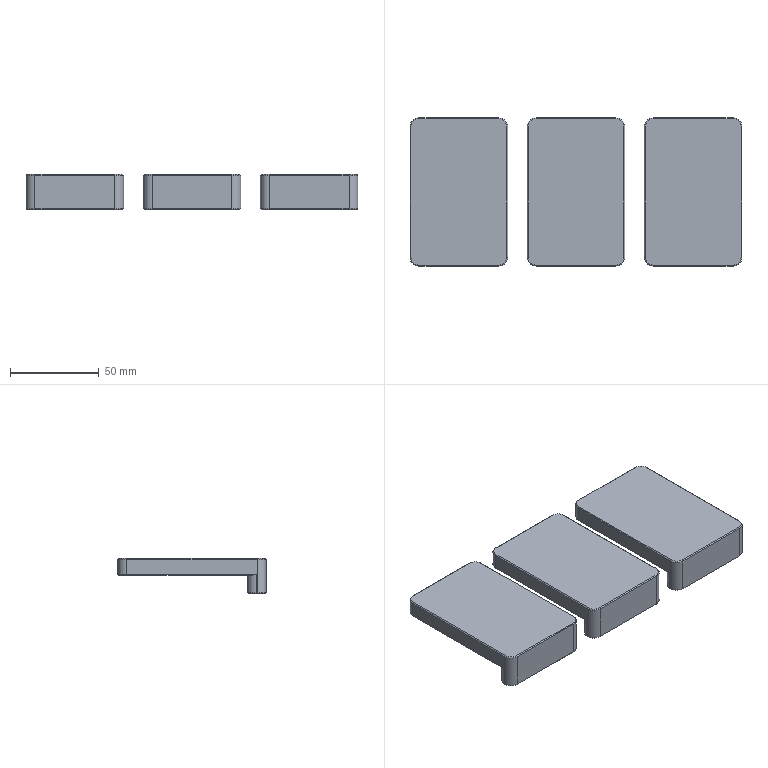NC program | NX | posted with a generic post | part box 187 x 83.5 x 20 mm
Lines 5413 to 5666 of 5666:
(ZLEVEL_PROFILE_COPY_1_COPY , TOOL : D10JING)
N10818 T14 M6
N10820 G54
N10822 G17 G0 G90 X33.89 Y39.594 S9500 M3
N10824 G43 Z30. H14
N10826 Z1.5
N10828 G94 G1 X34.613 Y41.399 Z1.398 F1000.
N10830 X35.728 Y43.09 Z1.292
N10832 X37.16 Y44.522 Z1.186
N10834 X38.851 Y45.637 Z1.08
N10836 X40.731 Y46.39 Z0.973
N10838 X42.725 Y46.75 Z0.867
N10840 X89.275 Z-1.572
N10842 X91.269 Y46.39 Z-1.678
N10844 X93.149 Y45.637 Z-1.785
N10846 X94.84 Y44.522 Z-1.891
N10848 X96.272 Y43.09 Z-1.997
N10850 X97.387 Y41.399 Z-2.103
N10852 X98.14 Y39.519 Z-2.209
N10854 X98.5 Y37.525 Z-2.315
N10856 Y-37.525 Z-6.249
N10858 X98.14 Y-39.519 Z-6.355
N10860 X97.387 Y-41.399 Z-6.461
N10862 X96.272 Y-43.09 Z-6.567
N10864 X94.84 Y-44.522 Z-6.673
N10866 X93.149 Y-45.637 Z-6.779
N10868 X91.269 Y-46.39 Z-6.886
N10870 X89.275 Y-46.75 Z-6.992
N10872 X42.725 Z-9.431
N10874 X40.731 Y-46.39 Z-9.537
N10876 X38.851 Y-45.637 Z-9.644
N10878 X37.16 Y-44.522 Z-9.75
N10880 X35.728 Y-43.09 Z-9.856
N10882 X34.613 Y-41.399 Z-9.962
N10884 X33.86 Y-39.519 Z-10.068
N10886 X33.5 Y-37.525 Z-10.174
N10888 Y37.525 Z-14.108
N10890 X33.86 Y39.519 Z-14.214
N10892 X34.613 Y41.399 Z-14.32
N10894 X35.728 Y43.09 Z-14.426
N10896 X37.16 Y44.522 Z-14.532
N10898 X38.851 Y45.637 Z-14.638
N10900 X40.731 Y46.39 Z-14.745
N10902 X42.725 Y46.75 Z-14.851
N10904 X89.275 Z-17.29
N10906 X91.269 Y46.39 Z-17.396
N10908 X93.149 Y45.637 Z-17.503
N10910 X94.84 Y44.522 Z-17.609
N10912 X96.272 Y43.09 Z-17.715
N10914 X97.387 Y41.399 Z-17.821
N10916 X98.14 Y39.519 Z-17.927
N10918 X98.5 Y37.525 Z-18.033
N10920 Y0. Z-20.
N10922 Y-36.75 F1200.
N10924 G2 X88.5 Y-46.75 R10.
N10926 G1 X43.5
N10928 G2 X33.5 Y-36.75 R10.
N10930 G1 Y36.75
N10932 G2 X43.5 Y46.75 R10.
N10934 G1 X88.5
N10936 G2 X98.5 Y36.75 R10.
N10938 G1 Y0.
N10940 G3 X99. Y-0.866 R1.
N10942 G1 X99.5 Y-1.155
N10944 Z-19.
N10946 G0 Z53.
N10948 X-33.89 Y-39.594
N10950 Z1.5
N10952 G1 X-34.613 Y-41.399 Z1.398 F1000.
N10954 X-35.728 Y-43.09 Z1.292
N10956 X-37.16 Y-44.522 Z1.186
N10958 X-38.851 Y-45.637 Z1.08
N10960 X-40.731 Y-46.39 Z0.973
N10962 X-42.725 Y-46.75 Z0.867
N10964 X-89.275 Z-1.572
N10966 X-91.269 Y-46.39 Z-1.678
N10968 X-93.149 Y-45.637 Z-1.785
N10970 X-94.84 Y-44.522 Z-1.891
N10972 X-96.272 Y-43.09 Z-1.997
N10974 X-97.387 Y-41.399 Z-2.103
N10976 X-98.14 Y-39.519 Z-2.209
N10978 X-98.5 Y-37.525 Z-2.315
N10980 Y37.525 Z-6.249
N10982 X-98.14 Y39.519 Z-6.355
N10984 X-97.387 Y41.399 Z-6.461
N10986 X-96.272 Y43.09 Z-6.567
N10988 X-94.84 Y44.522 Z-6.673
N10990 X-93.149 Y45.637 Z-6.779
N10992 X-91.269 Y46.39 Z-6.886
N10994 X-89.275 Y46.75 Z-6.992
N10996 X-42.725 Z-9.431
N10998 X-40.731 Y46.39 Z-9.537
N11000 X-38.851 Y45.637 Z-9.644
N11002 X-37.16 Y44.522 Z-9.75
N11004 X-35.728 Y43.09 Z-9.856
N11006 X-34.613 Y41.399 Z-9.962
N11008 X-33.86 Y39.519 Z-10.068
N11010 X-33.5 Y37.525 Z-10.174
N11012 Y-37.525 Z-14.108
N11014 X-33.86 Y-39.519 Z-14.214
N11016 X-34.613 Y-41.399 Z-14.32
N11018 X-35.728 Y-43.09 Z-14.426
N11020 X-37.16 Y-44.522 Z-14.532
N11022 X-38.851 Y-45.637 Z-14.638
N11024 X-40.731 Y-46.39 Z-14.745
N11026 X-42.725 Y-46.75 Z-14.851
N11028 X-89.275 Z-17.29
N11030 X-91.269 Y-46.39 Z-17.396
N11032 X-93.149 Y-45.637 Z-17.503
N11034 X-94.84 Y-44.522 Z-17.609
N11036 X-96.272 Y-43.09 Z-17.715
N11038 X-97.387 Y-41.399 Z-17.821
N11040 X-98.14 Y-39.519 Z-17.927
N11042 X-98.5 Y-37.525 Z-18.033
N11044 Y0. Z-20.
N11046 Y36.75 F1200.
N11048 G2 X-88.5 Y46.75 R10.
N11050 G1 X-43.5
N11052 G2 X-33.5 Y36.75 R10.
N11054 G1 Y-36.75
N11056 G2 X-43.5 Y-46.75 R10.
N11058 G1 X-88.5
N11060 G2 X-98.5 Y-36.75 R10.
N11062 G1 Y0.
N11064 G3 X-99. Y0.866 R1.
N11066 G1 X-99.5 Y1.155
N11068 Z-19.
N11070 G0 Z53.
N11072 X32.11 Y-39.594
N11074 Z1.5
N11076 G1 X31.387 Y-41.399 Z1.398 F1000.
N11078 X30.272 Y-43.09 Z1.292
N11080 X28.84 Y-44.522 Z1.186
N11082 X27.149 Y-45.637 Z1.08
N11084 X25.269 Y-46.39 Z0.973
N11086 X23.275 Y-46.75 Z0.867
N11088 X-23.275 Z-1.572
N11090 X-25.269 Y-46.39 Z-1.678
N11092 X-27.149 Y-45.637 Z-1.785
N11094 X-28.84 Y-44.522 Z-1.891
N11096 X-30.272 Y-43.09 Z-1.997
N11098 X-31.387 Y-41.399 Z-2.103
N11100 X-32.14 Y-39.519 Z-2.209
N11102 X-32.5 Y-37.525 Z-2.315
N11104 Y37.525 Z-6.249
N11106 X-32.14 Y39.519 Z-6.355
N11108 X-31.387 Y41.399 Z-6.461
N11110 X-30.272 Y43.09 Z-6.567
N11112 X-28.84 Y44.522 Z-6.673
N11114 X-27.149 Y45.637 Z-6.779
N11116 X-25.269 Y46.39 Z-6.886
N11118 X-23.275 Y46.75 Z-6.992
N11120 X23.275 Z-9.431
N11122 X25.269 Y46.39 Z-9.537
N11124 X27.149 Y45.637 Z-9.644
N11126 X28.84 Y44.522 Z-9.75
N11128 X30.272 Y43.09 Z-9.856
N11130 X31.387 Y41.399 Z-9.962
N11132 X32.14 Y39.519 Z-10.068
N11134 X32.5 Y37.525 Z-10.174
N11136 Y-37.525 Z-14.108
N11138 X32.14 Y-39.519 Z-14.214
N11140 X31.387 Y-41.399 Z-14.32
N11142 X30.272 Y-43.09 Z-14.426
N11144 X28.84 Y-44.522 Z-14.532
N11146 X27.149 Y-45.637 Z-14.638
N11148 X25.269 Y-46.39 Z-14.745
N11150 X23.275 Y-46.75 Z-14.851
N11152 X-23.275 Z-17.29
N11154 X-25.269 Y-46.39 Z-17.396
N11156 X-27.149 Y-45.637 Z-17.503
N11158 X-28.84 Y-44.522 Z-17.609
N11160 X-30.272 Y-43.09 Z-17.715
N11162 X-31.387 Y-41.399 Z-17.821
N11164 X-32.14 Y-39.519 Z-17.927
N11166 X-32.5 Y-37.525 Z-18.033
N11168 Y0. Z-20.
N11170 Y36.75 F1200.
N11172 G2 X-22.5 Y46.75 R10.
N11174 G1 X22.5
N11176 G2 X32.5 Y36.75 R10.
N11178 G1 Y-36.75
N11180 G2 X22.5 Y-46.75 R10.
N11182 G1 X-22.5
N11184 G2 X-32.5 Y-36.75 R10.
N11186 G1 Y0.
N11188 G3 X-33. Y0.866 R1.
N11190 G1 Z-19.
N11192 G0 Z30.
N11194 M5
(PLANAR_MILL_COPY_COPY_COPY_COPY , TOOL : D6A45)
N11196 T01 M6
N11198 G54
N11200 G17 G0 G90 X95.7 Y1.27 S9500 M3
N11202 G43 Z30. H1
N11204 Z0.
N11206 G94 G1 Z-1.5 F1250.
N11208 X95. Y0.866
N11210 G3 X94.5 Y0. R1.
N11212 G1 Y-36.75
N11214 G2 X88.5 Y-42.75 R6.
N11216 G1 X43.5
N11218 G2 X37.5 Y-36.75 R6.
N11220 G1 Y36.75
N11222 G2 X43.5 Y42.75 R6.
N11224 G1 X88.5
N11226 G2 X94.5 Y36.75 R6.
N11228 G1 Y0.
N11230 G3 X95. Y-0.866 R1.
N11232 G1 X95.7 Y-1.27
N11234 Z0.
N11236 G0 Z30.
N11238 X29.7 Y1.27
N11240 Z0.
N11242 G1 Z-1.5
N11244 X29. Y0.866
N11246 G3 X28.5 Y0. R1.
N11248 G1 Y-36.75
N11250 G2 X22.5 Y-42.75 R6.
N11252 G1 X-22.5
N11254 G2 X-28.5 Y-36.75 R6.
N11256 G1 Y36.75
N11258 G2 X-22.5 Y42.75 R6.
N11260 G1 X22.5
N11262 G2 X28.5 Y36.75 R6.
N11264 G1 Y0.
N11266 G3 X29. Y-0.866 R1.
N11268 G1 X29.7 Y-1.27
N11270 Z0.
N11272 G0 Z30.
N11274 X-95.7
N11276 Z0.
N11278 G1 Z-1.5
N11280 X-95. Y-0.866
N11282 G3 X-94.5 Y0. R1.
N11284 G1 Y36.75
N11286 G2 X-88.5 Y42.75 R6.
N11288 G1 X-43.5
N11290 G2 X-37.5 Y36.75 R6.
N11292 G1 Y-36.75
N11294 G2 X-43.5 Y-42.75 R6.
N11296 G1 X-88.5
N11298 G2 X-94.5 Y-36.75 R6.
N11300 G1 Y0.
N11302 G3 X-95. Y0.866 R1.
N11304 G1 X-95.7 Y1.27
N11306 Z0.
N11308 G0 Z30.
N11310 M5
N11312 M2